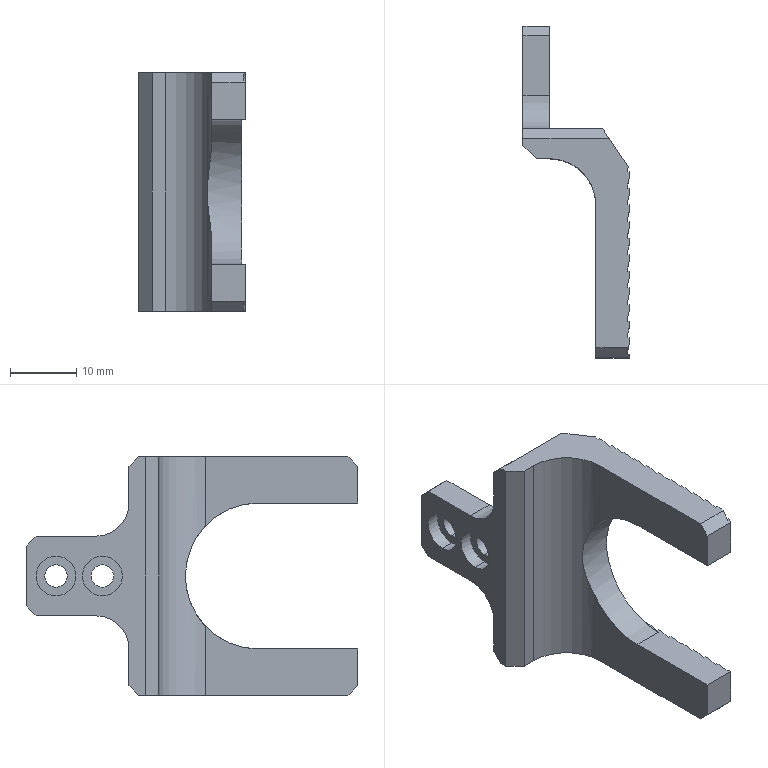Part | STEP file | 0-19 Finger 2 | 1 solid | 110 faces | box 16 x 50 x 36 mm | volume 5757 mm3 | plane 98 | cylinder 12 | commonest cylinder face diameters 3.4 x4 6 x4 10 x2 14 x1 22 x1